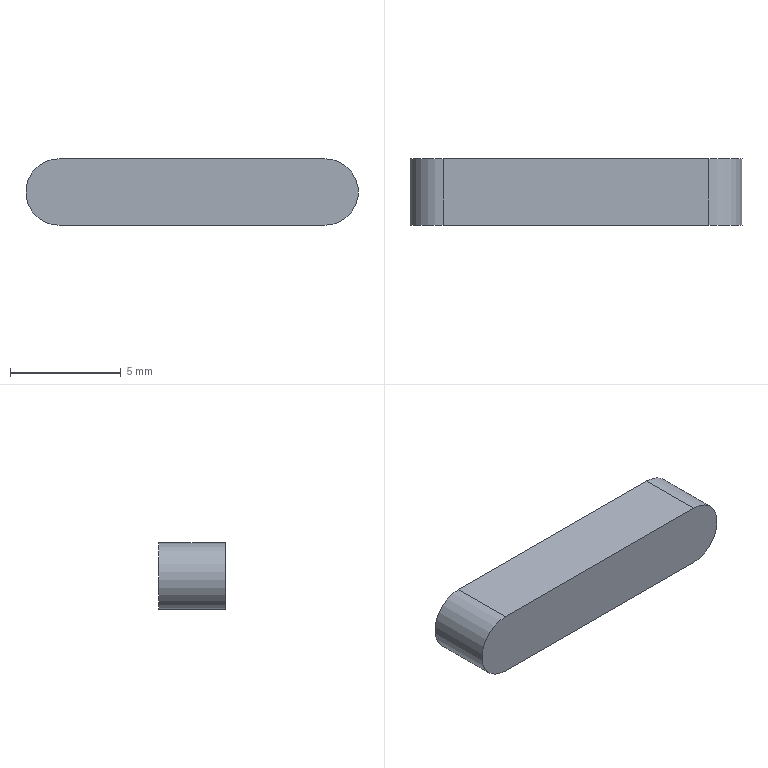Part | NX | features BREP 1 | 1 solid | 6 faces | box 15 x 3 x 3 mm | volume 129.206 mm3 | plane 4 | cylinder 2 | commonest cylinder face diameters 3 x2
STEP:
#1=CARTESIAN_POINT('',(0.,0.,-1.5));
#2=VERTEX_POINT('',#1);
#3=CARTESIAN_POINT('',(0.,0.,1.5));
#4=VERTEX_POINT('',#3);
#5=CARTESIAN_POINT('',(0.,0.,0.));
#6=DIRECTION('',(0.,1.,0.));
#7=DIRECTION('',(0.,0.,1.));
#8=AXIS2_PLACEMENT_3D('',#5,#6,#7);
#9=CIRCLE('',#8,1.5);
#10=EDGE_CURVE('',#2,#4,#9,.T.);
#11=ORIENTED_EDGE('',*,*,#10,.T.);
#12=CARTESIAN_POINT('',(0.,3.,1.5));
#13=VERTEX_POINT('',#12);
#14=CARTESIAN_POINT('',(0.,3.,1.5));
#15=DIRECTION('',(0.,-1.,0.));
#16=VECTOR('',#15,1000.);
#17=LINE('',#14,#16);
#18=EDGE_CURVE('',#13,#4,#17,.T.);
#19=ORIENTED_EDGE('',*,*,#18,.F.);
#20=CARTESIAN_POINT('',(0.,3.,-1.5));
#21=VERTEX_POINT('',#20);
#22=CARTESIAN_POINT('',(0.,3.,0.));
#23=DIRECTION('',(0.,1.,0.));
#24=DIRECTION('',(0.,0.,1.));
#25=AXIS2_PLACEMENT_3D('',#22,#23,#24);
#26=CIRCLE('',#25,1.5);
#27=EDGE_CURVE('',#21,#13,#26,.T.);
#28=ORIENTED_EDGE('',*,*,#27,.F.);
#29=CARTESIAN_POINT('',(0.,3.,-1.5));
#30=DIRECTION('',(0.,-1.,0.));
#31=VECTOR('',#30,1000.);
#32=LINE('',#29,#31);
#33=EDGE_CURVE('',#21,#2,#32,.T.);
#34=ORIENTED_EDGE('',*,*,#33,.T.);
#35=EDGE_LOOP('',(#11,#19,#28,#34));
#36=FACE_BOUND('',#35,.T.);
#37=CARTESIAN_POINT('',(0.,3.,0.));
#38=DIRECTION('',(0.,-1.,0.));
#39=DIRECTION('',(0.,0.,1.));
#40=AXIS2_PLACEMENT_3D('',#37,#38,#39);
#41=CYLINDRICAL_SURFACE('',#40,1.5);
#42=ADVANCED_FACE('',(#36),#41,.T.);
#43=CARTESIAN_POINT('',(12.,0.,1.5));
#44=VERTEX_POINT('',#43);
#45=CARTESIAN_POINT('',(0.,0.,1.5));
#46=DIRECTION('',(1.,0.,0.));
#47=VECTOR('',#46,1000.);
#48=LINE('',#45,#47);
#49=EDGE_CURVE('',#4,#44,#48,.T.);
#50=ORIENTED_EDGE('',*,*,#49,.T.);
#51=CARTESIAN_POINT('',(12.,3.,1.5));
#52=VERTEX_POINT('',#51);
#53=CARTESIAN_POINT('',(12.,3.,1.5));
#54=DIRECTION('',(0.,-1.,0.));
#55=VECTOR('',#54,1000.);
#56=LINE('',#53,#55);
#57=EDGE_CURVE('',#52,#44,#56,.T.);
#58=ORIENTED_EDGE('',*,*,#57,.F.);
#59=CARTESIAN_POINT('',(0.,3.,1.5));
#60=DIRECTION('',(1.,0.,0.));
#61=VECTOR('',#60,1000.);
#62=LINE('',#59,#61);
#63=EDGE_CURVE('',#13,#52,#62,.T.);
#64=ORIENTED_EDGE('',*,*,#63,.F.);
#65=ORIENTED_EDGE('',*,*,#18,.T.);
#66=EDGE_LOOP('',(#50,#58,#64,#65));
#67=FACE_BOUND('',#66,.T.);
#68=CARTESIAN_POINT('',(0.,3.,1.5));
#69=DIRECTION('',(0.,0.,-1.));
#70=DIRECTION('',(0.,1.,0.));
#71=AXIS2_PLACEMENT_3D('',#68,#69,#70);
#72=PLANE('',#71);
#73=ADVANCED_FACE('',(#67),#72,.F.);
#74=CARTESIAN_POINT('',(12.,0.,-1.5));
#75=VERTEX_POINT('',#74);
#76=CARTESIAN_POINT('',(12.,0.,0.));
#77=DIRECTION('',(0.,1.,0.));
#78=DIRECTION('',(0.,0.,1.));
#79=AXIS2_PLACEMENT_3D('',#76,#77,#78);
#80=CIRCLE('',#79,1.5);
#81=EDGE_CURVE('',#44,#75,#80,.T.);
#82=ORIENTED_EDGE('',*,*,#81,.T.);
#83=CARTESIAN_POINT('',(12.,3.,-1.5));
#84=VERTEX_POINT('',#83);
#85=CARTESIAN_POINT('',(12.,3.,-1.5));
#86=DIRECTION('',(0.,-1.,0.));
#87=VECTOR('',#86,1000.);
#88=LINE('',#85,#87);
#89=EDGE_CURVE('',#84,#75,#88,.T.);
#90=ORIENTED_EDGE('',*,*,#89,.F.);
#91=CARTESIAN_POINT('',(12.,3.,0.));
#92=DIRECTION('',(0.,1.,0.));
#93=DIRECTION('',(0.,0.,1.));
#94=AXIS2_PLACEMENT_3D('',#91,#92,#93);
#95=CIRCLE('',#94,1.5);
#96=EDGE_CURVE('',#52,#84,#95,.T.);
#97=ORIENTED_EDGE('',*,*,#96,.F.);
#98=ORIENTED_EDGE('',*,*,#57,.T.);
#99=EDGE_LOOP('',(#82,#90,#97,#98));
#100=FACE_BOUND('',#99,.T.);
#101=CARTESIAN_POINT('',(12.,3.,0.));
#102=DIRECTION('',(0.,-1.,0.));
#103=DIRECTION('',(0.,0.,1.));
#104=AXIS2_PLACEMENT_3D('',#101,#102,#103);
#105=CYLINDRICAL_SURFACE('',#104,1.5);
#106=ADVANCED_FACE('',(#100),#105,.T.);
#107=CARTESIAN_POINT('',(12.,0.,-1.5));
#108=DIRECTION('',(-1.,0.,0.));
#109=VECTOR('',#108,1000.);
#110=LINE('',#107,#109);
#111=EDGE_CURVE('',#75,#2,#110,.T.);
#112=ORIENTED_EDGE('',*,*,#111,.T.);
#113=ORIENTED_EDGE('',*,*,#33,.F.);
#114=CARTESIAN_POINT('',(12.,3.,-1.5));
#115=DIRECTION('',(-1.,0.,0.));
#116=VECTOR('',#115,1000.);
#117=LINE('',#114,#116);
#118=EDGE_CURVE('',#84,#21,#117,.T.);
#119=ORIENTED_EDGE('',*,*,#118,.F.);
#120=ORIENTED_EDGE('',*,*,#89,.T.);
#121=EDGE_LOOP('',(#112,#113,#119,#120));
#122=FACE_BOUND('',#121,.T.);
#123=CARTESIAN_POINT('',(12.,3.,-1.5));
#124=DIRECTION('',(0.,0.,1.));
#125=DIRECTION('',(0.,1.,0.));
#126=AXIS2_PLACEMENT_3D('',#123,#124,#125);
#127=PLANE('',#126);
#128=ADVANCED_FACE('',(#122),#127,.F.);
#129=ORIENTED_EDGE('',*,*,#27,.T.);
#130=ORIENTED_EDGE('',*,*,#63,.T.);
#131=ORIENTED_EDGE('',*,*,#96,.T.);
#132=ORIENTED_EDGE('',*,*,#118,.T.);
#133=EDGE_LOOP('',(#129,#130,#131,#132));
#134=FACE_BOUND('',#133,.T.);
#135=CARTESIAN_POINT('',(0.,3.,0.));
#136=DIRECTION('',(0.,1.,0.));
#137=DIRECTION('',(0.,0.,1.));
#138=AXIS2_PLACEMENT_3D('',#135,#136,#137);
#139=PLANE('',#138);
#140=ADVANCED_FACE('',(#134),#139,.T.);
#141=ORIENTED_EDGE('',*,*,#10,.F.);
#142=ORIENTED_EDGE('',*,*,#111,.F.);
#143=ORIENTED_EDGE('',*,*,#81,.F.);
#144=ORIENTED_EDGE('',*,*,#49,.F.);
#145=EDGE_LOOP('',(#141,#142,#143,#144));
#146=FACE_BOUND('',#145,.T.);
#147=CARTESIAN_POINT('',(0.,0.,0.));
#148=DIRECTION('',(0.,1.,0.));
#149=DIRECTION('',(0.,0.,1.));
#150=AXIS2_PLACEMENT_3D('',#147,#148,#149);
#151=PLANE('',#150);
#152=ADVANCED_FACE('',(#146),#151,.F.);
#153=CLOSED_SHELL('',(#42,#73,#106,#128,#140,#152));
#154=MANIFOLD_SOLID_BREP('',#153);
#155=(LENGTH_UNIT()NAMED_UNIT(*)SI_UNIT(.MILLI.,.METRE.));
#156=UNCERTAINTY_MEASURE_WITH_UNIT(LENGTH_MEASURE(0.00001),#155,'','');
#157=(NAMED_UNIT(*)PLANE_ANGLE_UNIT()SI_UNIT($,.RADIAN.));
#158=(NAMED_UNIT(*)SI_UNIT($,.STERADIAN.)SOLID_ANGLE_UNIT());
#159=(GEOMETRIC_REPRESENTATION_CONTEXT(3)GLOBAL_UNCERTAINTY_ASSIGNED_CONTEXT((#156))GLOBAL_UNIT_ASSIGNED_CONTEXT((#155,#157,#158))REPRESENTATION_CONTEXT('',''));
#160=ADVANCED_BREP_SHAPE_REPRESENTATION('',(#154),#159);